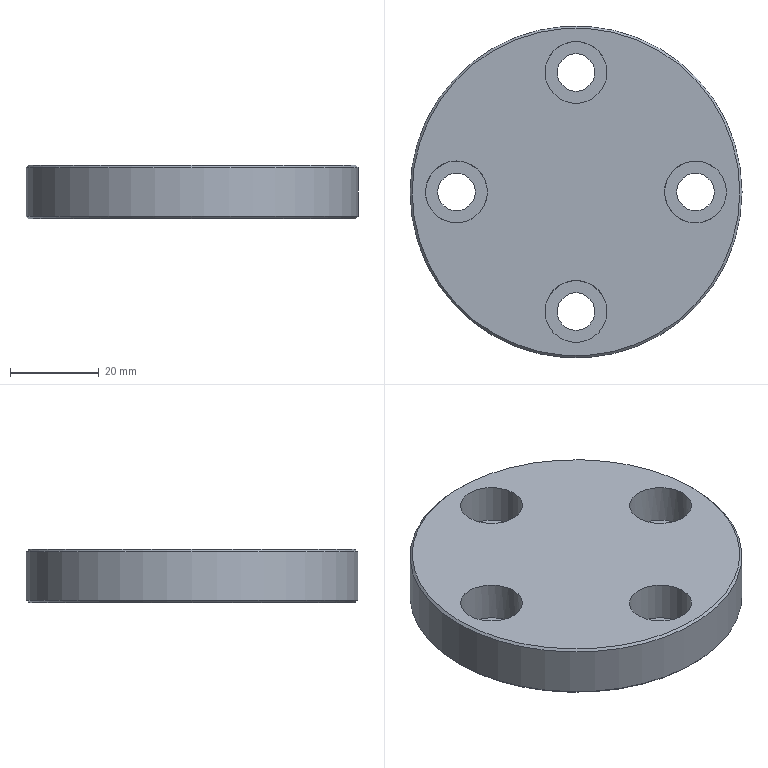Part | STEP file | solid 99 | 1 solid | 17 faces | box 75 x 75 x 12 mm | volume 46733 mm3 | cylinder 9 | plane 6 | cone 2 | commonest cylinder face diameters 8.5 x4 14 x4 75 x1